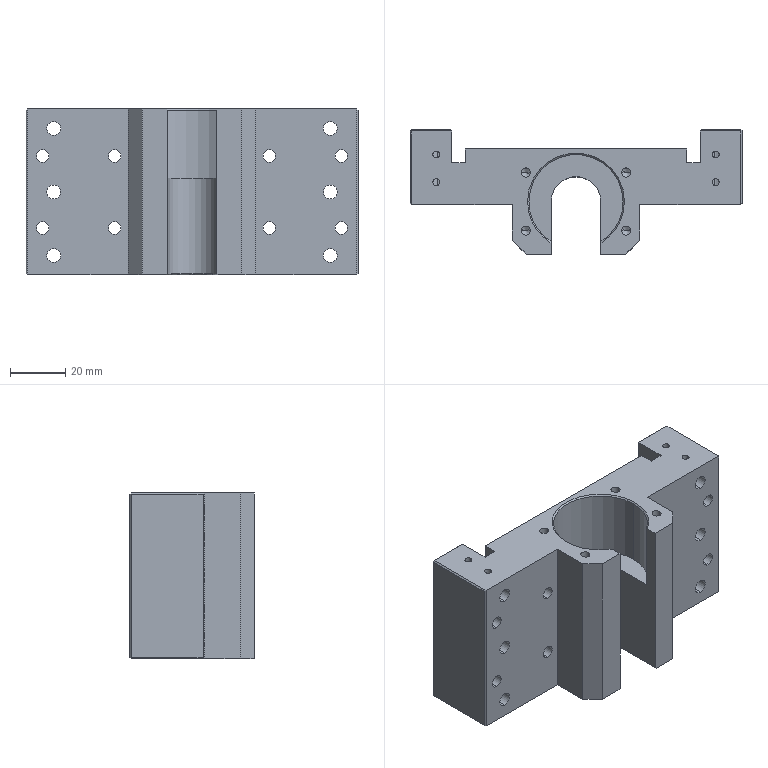Part | STEP file | 1 solid | 148 faces | box 120 x 45 x 60 mm | volume 150732 mm3 | cylinder 72 | plane 52 | cone 24 | commonest cylinder face diameters 2.5 x16 4.5 x16 8 x16 5 x12 3.3 x8 34 x3